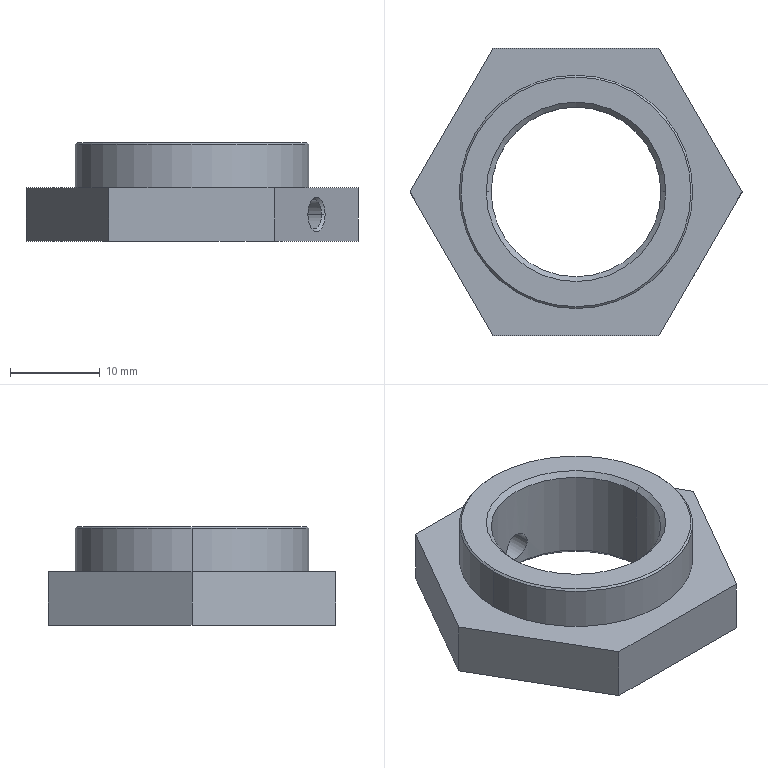Part | STEP file | BKN51-M20^Drive roller assembly | 1 solid | 27 faces | box 37 x 32.043 x 11 mm | volume 4769 mm3 | cone 10 | plane 9 | cylinder 8 | commonest cylinder face diameters 3.242 x4 18.917 x2 26 x2